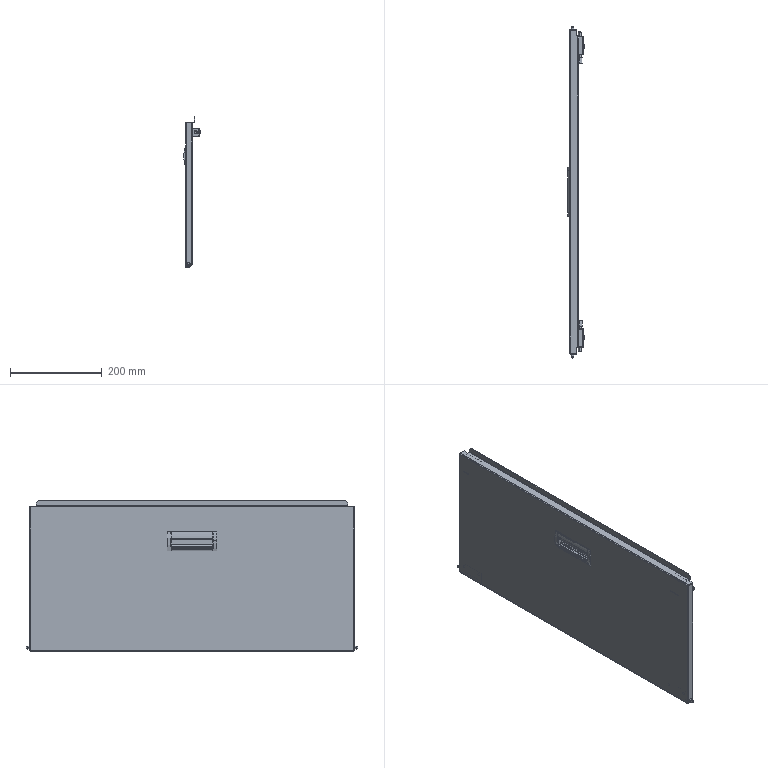Part | SolidWorks | 16 solids | 429 faces | box 35.649 x 724 x 329 mm | volume 451406 mm3 | plane 243 | cylinder 174 | cone 8 | torus 4 | commonest cylinder face diameters 1 x18 2.5 x16 3.2 x16 0.6 x14 7 x13 2 x8